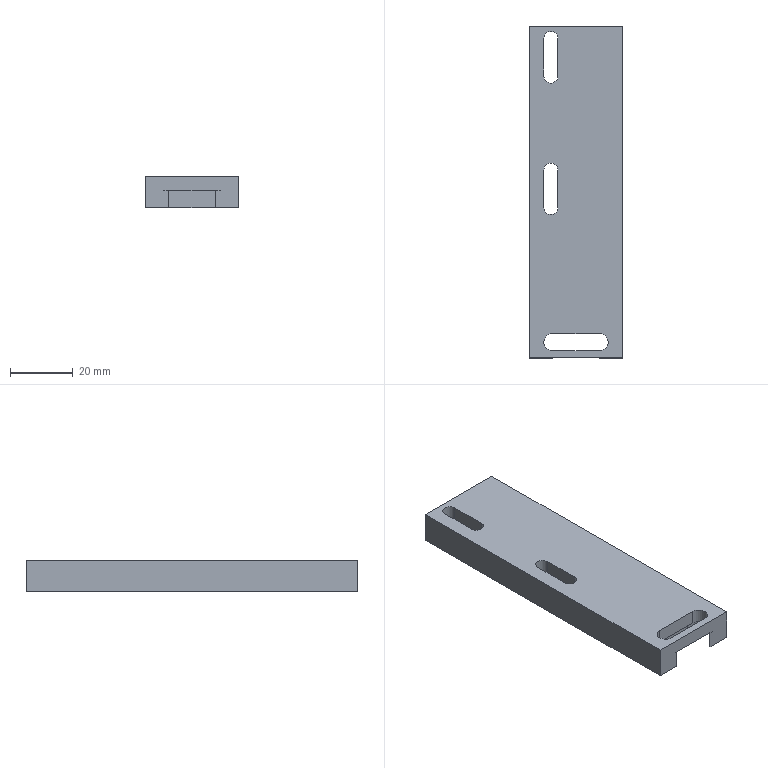Part | NX | 1 solid | 22 faces | box 30 x 106 x 10 mm | volume 28667 mm3 | plane 14 | cylinder 8 | commonest cylinder face diameters 4.5 x4 5.5 x2 10 x2
STEP:
#1=CARTESIAN_POINT('',(-10.25,49.,0.));
#2=VERTEX_POINT('',#1);
#3=CARTESIAN_POINT('',(-10.25,37.,0.));
#4=VERTEX_POINT('',#3);
#5=CARTESIAN_POINT('',(-10.25,0.,0.));
#6=DIRECTION('',(0.,-1.,0.));
#7=VECTOR('',#6,1000.);
#8=LINE('',#5,#7);
#9=EDGE_CURVE('',#2,#4,#8,.T.);
#10=ORIENTED_EDGE('',*,*,#9,.T.);
#11=CARTESIAN_POINT('',(-5.75,37.,0.));
#12=VERTEX_POINT('',#11);
#13=CARTESIAN_POINT('',(-8.,37.,0.));
#14=DIRECTION('',(0.,0.,1.));
#15=DIRECTION('',(1.,0.,0.));
#16=AXIS2_PLACEMENT_3D('',#13,#14,#15);
#17=CIRCLE('',#16,2.25);
#18=EDGE_CURVE('',#4,#12,#17,.T.);
#19=ORIENTED_EDGE('',*,*,#18,.T.);
#20=CARTESIAN_POINT('',(-5.75,49.,0.));
#21=VERTEX_POINT('',#20);
#22=CARTESIAN_POINT('',(-5.75,0.,0.));
#23=DIRECTION('',(0.,1.,0.));
#24=VECTOR('',#23,1000.);
#25=LINE('',#22,#24);
#26=EDGE_CURVE('',#12,#21,#25,.T.);
#27=ORIENTED_EDGE('',*,*,#26,.T.);
#28=CARTESIAN_POINT('',(-8.,49.,0.));
#29=DIRECTION('',(0.,0.,1.));
#30=DIRECTION('',(-1.,0.,0.));
#31=AXIS2_PLACEMENT_3D('',#28,#29,#30);
#32=CIRCLE('',#31,2.25);
#33=EDGE_CURVE('',#21,#2,#32,.T.);
#34=ORIENTED_EDGE('',*,*,#33,.T.);
#35=EDGE_LOOP('',(#10,#19,#27,#34));
#36=FACE_BOUND('',#35,.T.);
#37=CARTESIAN_POINT('',(-10.25,-5.,0.));
#38=VERTEX_POINT('',#37);
#39=CARTESIAN_POINT('',(-5.75,-5.,0.));
#40=VERTEX_POINT('',#39);
#41=CARTESIAN_POINT('',(-8.,-5.,0.));
#42=DIRECTION('',(0.,0.,1.));
#43=DIRECTION('',(1.,0.,0.));
#44=AXIS2_PLACEMENT_3D('',#41,#42,#43);
#45=CIRCLE('',#44,2.25);
#46=EDGE_CURVE('',#38,#40,#45,.T.);
#47=ORIENTED_EDGE('',*,*,#46,.T.);
#48=CARTESIAN_POINT('',(-5.75,7.,0.));
#49=VERTEX_POINT('',#48);
#50=CARTESIAN_POINT('',(-5.75,-2.5,0.));
#51=DIRECTION('',(0.,1.,0.));
#52=VECTOR('',#51,1000.);
#53=LINE('',#50,#52);
#54=EDGE_CURVE('',#40,#49,#53,.T.);
#55=ORIENTED_EDGE('',*,*,#54,.T.);
#56=CARTESIAN_POINT('',(-10.25,7.,0.));
#57=VERTEX_POINT('',#56);
#58=CARTESIAN_POINT('',(-8.,7.,0.));
#59=DIRECTION('',(0.,0.,1.));
#60=DIRECTION('',(-1.,0.,0.));
#61=AXIS2_PLACEMENT_3D('',#58,#59,#60);
#62=CIRCLE('',#61,2.25);
#63=EDGE_CURVE('',#49,#57,#62,.T.);
#64=ORIENTED_EDGE('',*,*,#63,.T.);
#65=CARTESIAN_POINT('',(-10.25,3.5,0.));
#66=DIRECTION('',(0.,-1.,0.));
#67=VECTOR('',#66,1000.);
#68=LINE('',#65,#67);
#69=EDGE_CURVE('',#57,#38,#68,.T.);
#70=ORIENTED_EDGE('',*,*,#69,.T.);
#71=EDGE_LOOP('',(#47,#55,#64,#70));
#72=FACE_BOUND('',#71,.T.);
#73=CARTESIAN_POINT('',(-7.5,-43.,0.));
#74=VERTEX_POINT('',#73);
#75=CARTESIAN_POINT('',(-7.5,-53.,0.));
#76=VERTEX_POINT('',#75);
#77=CARTESIAN_POINT('',(-7.5,-48.,0.));
#78=DIRECTION('',(0.,0.,1.));
#79=DIRECTION('',(0.,-1.,0.));
#80=AXIS2_PLACEMENT_3D('',#77,#78,#79);
#81=CIRCLE('',#80,5.);
#82=EDGE_CURVE('',#74,#76,#81,.T.);
#83=ORIENTED_EDGE('',*,*,#82,.T.);
#84=CARTESIAN_POINT('',(-15.,-53.,0.));
#85=VERTEX_POINT('',#84);
#86=CARTESIAN_POINT('',(-15.,-53.,0.));
#87=DIRECTION('',(1.,0.,0.));
#88=VECTOR('',#87,1000.);
#89=LINE('',#86,#88);
#90=EDGE_CURVE('',#85,#76,#89,.T.);
#91=ORIENTED_EDGE('',*,*,#90,.F.);
#92=CARTESIAN_POINT('',(-15.,53.,0.));
#93=VERTEX_POINT('',#92);
#94=CARTESIAN_POINT('',(-15.,53.,0.));
#95=DIRECTION('',(0.,-1.,0.));
#96=VECTOR('',#95,1000.);
#97=LINE('',#94,#96);
#98=EDGE_CURVE('',#93,#85,#97,.T.);
#99=ORIENTED_EDGE('',*,*,#98,.F.);
#100=CARTESIAN_POINT('',(15.,53.,0.));
#101=VERTEX_POINT('',#100);
#102=CARTESIAN_POINT('',(15.,53.,0.));
#103=DIRECTION('',(-1.,0.,0.));
#104=VECTOR('',#103,1000.);
#105=LINE('',#102,#104);
#106=EDGE_CURVE('',#101,#93,#105,.T.);
#107=ORIENTED_EDGE('',*,*,#106,.F.);
#108=CARTESIAN_POINT('',(15.,-53.,0.));
#109=VERTEX_POINT('',#108);
#110=CARTESIAN_POINT('',(15.,-53.,0.));
#111=DIRECTION('',(0.,1.,0.));
#112=VECTOR('',#111,1000.);
#113=LINE('',#110,#112);
#114=EDGE_CURVE('',#109,#101,#113,.T.);
#115=ORIENTED_EDGE('',*,*,#114,.F.);
#116=CARTESIAN_POINT('',(7.5,-53.,0.));
#117=VERTEX_POINT('',#116);
#118=CARTESIAN_POINT('',(-15.,-53.,0.));
#119=DIRECTION('',(1.,0.,0.));
#120=VECTOR('',#119,1000.);
#121=LINE('',#118,#120);
#122=EDGE_CURVE('',#117,#109,#121,.T.);
#123=ORIENTED_EDGE('',*,*,#122,.F.);
#124=CARTESIAN_POINT('',(7.5,-43.,0.));
#125=VERTEX_POINT('',#124);
#126=CARTESIAN_POINT('',(7.5,-48.,0.));
#127=DIRECTION('',(0.,0.,1.));
#128=DIRECTION('',(0.,1.,0.));
#129=AXIS2_PLACEMENT_3D('',#126,#127,#128);
#130=CIRCLE('',#129,5.);
#131=EDGE_CURVE('',#117,#125,#130,.T.);
#132=ORIENTED_EDGE('',*,*,#131,.T.);
#133=CARTESIAN_POINT('',(3.75,-43.,0.));
#134=DIRECTION('',(-1.,0.,0.));
#135=VECTOR('',#134,1000.);
#136=LINE('',#133,#135);
#137=EDGE_CURVE('',#125,#74,#136,.T.);
#138=ORIENTED_EDGE('',*,*,#137,.T.);
#139=EDGE_LOOP('',(#83,#91,#99,#107,#115,#123,#132,#138));
#140=FACE_BOUND('',#139,.T.);
#141=CARTESIAN_POINT('',(0.,0.,0.));
#142=DIRECTION('',(0.,0.,1.));
#143=DIRECTION('',(1.,0.,0.));
#144=AXIS2_PLACEMENT_3D('',#141,#142,#143);
#145=PLANE('',#144);
#146=ADVANCED_FACE('',(#36,#72,#140),#145,.F.);
#147=CARTESIAN_POINT('',(-10.25,37.,10.));
#148=VERTEX_POINT('',#147);
#149=CARTESIAN_POINT('',(-10.25,49.,10.));
#150=VERTEX_POINT('',#149);
#151=CARTESIAN_POINT('',(-10.25,0.,10.));
#152=DIRECTION('',(0.,1.,0.));
#153=VECTOR('',#152,1000.);
#154=LINE('',#151,#153);
#155=EDGE_CURVE('',#148,#150,#154,.T.);
#156=ORIENTED_EDGE('',*,*,#155,.T.);
#157=CARTESIAN_POINT('',(-5.75,49.,10.));
#158=VERTEX_POINT('',#157);
#159=CARTESIAN_POINT('',(-8.,49.,10.));
#160=DIRECTION('',(0.,0.,-1.));
#161=DIRECTION('',(-1.,0.,0.));
#162=AXIS2_PLACEMENT_3D('',#159,#160,#161);
#163=CIRCLE('',#162,2.25);
#164=EDGE_CURVE('',#150,#158,#163,.T.);
#165=ORIENTED_EDGE('',*,*,#164,.T.);
#166=CARTESIAN_POINT('',(-5.75,37.,10.));
#167=VERTEX_POINT('',#166);
#168=CARTESIAN_POINT('',(-5.75,0.,10.));
#169=DIRECTION('',(0.,-1.,0.));
#170=VECTOR('',#169,1000.);
#171=LINE('',#168,#170);
#172=EDGE_CURVE('',#158,#167,#171,.T.);
#173=ORIENTED_EDGE('',*,*,#172,.T.);
#174=CARTESIAN_POINT('',(-8.,37.,10.));
#175=DIRECTION('',(0.,0.,-1.));
#176=DIRECTION('',(1.,0.,0.));
#177=AXIS2_PLACEMENT_3D('',#174,#175,#176);
#178=CIRCLE('',#177,2.25);
#179=EDGE_CURVE('',#167,#148,#178,.T.);
#180=ORIENTED_EDGE('',*,*,#179,.T.);
#181=EDGE_LOOP('',(#156,#165,#173,#180));
#182=FACE_BOUND('',#181,.T.);
#183=CARTESIAN_POINT('',(-5.75,-5.,10.));
#184=VERTEX_POINT('',#183);
#185=CARTESIAN_POINT('',(-10.25,-5.,10.));
#186=VERTEX_POINT('',#185);
#187=CARTESIAN_POINT('',(-8.,-5.,10.));
#188=DIRECTION('',(0.,0.,-1.));
#189=DIRECTION('',(1.,0.,0.));
#190=AXIS2_PLACEMENT_3D('',#187,#188,#189);
#191=CIRCLE('',#190,2.25);
#192=EDGE_CURVE('',#184,#186,#191,.T.);
#193=ORIENTED_EDGE('',*,*,#192,.T.);
#194=CARTESIAN_POINT('',(-10.25,7.,10.));
#195=VERTEX_POINT('',#194);
#196=CARTESIAN_POINT('',(-10.25,3.5,10.));
#197=DIRECTION('',(0.,1.,0.));
#198=VECTOR('',#197,1000.);
#199=LINE('',#196,#198);
#200=EDGE_CURVE('',#186,#195,#199,.T.);
#201=ORIENTED_EDGE('',*,*,#200,.T.);
#202=CARTESIAN_POINT('',(-5.75,7.,10.));
#203=VERTEX_POINT('',#202);
#204=CARTESIAN_POINT('',(-8.,7.,10.));
#205=DIRECTION('',(0.,0.,-1.));
#206=DIRECTION('',(-1.,0.,0.));
#207=AXIS2_PLACEMENT_3D('',#204,#205,#206);
#208=CIRCLE('',#207,2.25);
#209=EDGE_CURVE('',#195,#203,#208,.T.);
#210=ORIENTED_EDGE('',*,*,#209,.T.);
#211=CARTESIAN_POINT('',(-5.75,-2.5,10.));
#212=DIRECTION('',(0.,-1.,0.));
#213=VECTOR('',#212,1000.);
#214=LINE('',#211,#213);
#215=EDGE_CURVE('',#203,#184,#214,.T.);
#216=ORIENTED_EDGE('',*,*,#215,.T.);
#217=EDGE_LOOP('',(#193,#201,#210,#216));
#218=FACE_BOUND('',#217,.T.);
#219=CARTESIAN_POINT('',(-7.5,-45.25,10.));
#220=VERTEX_POINT('',#219);
#221=CARTESIAN_POINT('',(7.5,-45.25,10.));
#222=VERTEX_POINT('',#221);
#223=CARTESIAN_POINT('',(3.75,-45.25,10.));
#224=DIRECTION('',(1.,0.,0.));
#225=VECTOR('',#224,1000.);
#226=LINE('',#223,#225);
#227=EDGE_CURVE('',#220,#222,#226,.T.);
#228=ORIENTED_EDGE('',*,*,#227,.T.);
#229=CARTESIAN_POINT('',(7.5,-50.75,10.));
#230=VERTEX_POINT('',#229);
#231=CARTESIAN_POINT('',(7.5,-48.,10.));
#232=DIRECTION('',(0.,0.,-1.));
#233=DIRECTION('',(0.,1.,0.));
#234=AXIS2_PLACEMENT_3D('',#231,#232,#233);
#235=CIRCLE('',#234,2.75);
#236=EDGE_CURVE('',#222,#230,#235,.T.);
#237=ORIENTED_EDGE('',*,*,#236,.T.);
#238=CARTESIAN_POINT('',(-7.5,-50.75,10.));
#239=VERTEX_POINT('',#238);
#240=CARTESIAN_POINT('',(-3.75,-50.75,10.));
#241=DIRECTION('',(-1.,0.,0.));
#242=VECTOR('',#241,1000.);
#243=LINE('',#240,#242);
#244=EDGE_CURVE('',#230,#239,#243,.T.);
#245=ORIENTED_EDGE('',*,*,#244,.T.);
#246=CARTESIAN_POINT('',(-7.5,-48.,10.));
#247=DIRECTION('',(0.,0.,-1.));
#248=DIRECTION('',(0.,-1.,0.));
#249=AXIS2_PLACEMENT_3D('',#246,#247,#248);
#250=CIRCLE('',#249,2.75);
#251=EDGE_CURVE('',#239,#220,#250,.T.);
#252=ORIENTED_EDGE('',*,*,#251,.T.);
#253=EDGE_LOOP('',(#228,#237,#245,#252));
#254=FACE_BOUND('',#253,.T.);
#255=CARTESIAN_POINT('',(15.,-53.,10.));
#256=VERTEX_POINT('',#255);
#257=CARTESIAN_POINT('',(15.,53.,10.));
#258=VERTEX_POINT('',#257);
#259=CARTESIAN_POINT('',(15.,-53.,10.));
#260=DIRECTION('',(0.,1.,0.));
#261=VECTOR('',#260,1000.);
#262=LINE('',#259,#261);
#263=EDGE_CURVE('',#256,#258,#262,.T.);
#264=ORIENTED_EDGE('',*,*,#263,.T.);
#265=CARTESIAN_POINT('',(-15.,53.,10.));
#266=VERTEX_POINT('',#265);
#267=CARTESIAN_POINT('',(15.,53.,10.));
#268=DIRECTION('',(-1.,0.,0.));
#269=VECTOR('',#268,1000.);
#270=LINE('',#267,#269);
#271=EDGE_CURVE('',#258,#266,#270,.T.);
#272=ORIENTED_EDGE('',*,*,#271,.T.);
#273=CARTESIAN_POINT('',(-15.,-53.,10.));
#274=VERTEX_POINT('',#273);
#275=CARTESIAN_POINT('',(-15.,53.,10.));
#276=DIRECTION('',(0.,-1.,0.));
#277=VECTOR('',#276,1000.);
#278=LINE('',#275,#277);
#279=EDGE_CURVE('',#266,#274,#278,.T.);
#280=ORIENTED_EDGE('',*,*,#279,.T.);
#281=CARTESIAN_POINT('',(-15.,-53.,10.));
#282=DIRECTION('',(1.,0.,0.));
#283=VECTOR('',#282,1000.);
#284=LINE('',#281,#283);
#285=EDGE_CURVE('',#274,#256,#284,.T.);
#286=ORIENTED_EDGE('',*,*,#285,.T.);
#287=EDGE_LOOP('',(#264,#272,#280,#286));
#288=FACE_BOUND('',#287,.T.);
#289=CARTESIAN_POINT('',(0.,0.,10.));
#290=DIRECTION('',(0.,0.,1.));
#291=DIRECTION('',(1.,0.,0.));
#292=AXIS2_PLACEMENT_3D('',#289,#290,#291);
#293=PLANE('',#292);
#294=ADVANCED_FACE('',(#182,#218,#254,#288),#293,.T.);
#295=ORIENTED_EDGE('',*,*,#114,.T.);
#296=CARTESIAN_POINT('',(15.,53.,0.));
#297=DIRECTION('',(0.,0.,1.));
#298=VECTOR('',#297,1000.);
#299=LINE('',#296,#298);
#300=EDGE_CURVE('',#101,#258,#299,.T.);
#301=ORIENTED_EDGE('',*,*,#300,.T.);
#302=ORIENTED_EDGE('',*,*,#263,.F.);
#303=CARTESIAN_POINT('',(15.,-53.,0.));
#304=DIRECTION('',(0.,0.,1.));
#305=VECTOR('',#304,1000.);
#306=LINE('',#303,#305);
#307=EDGE_CURVE('',#109,#256,#306,.T.);
#308=ORIENTED_EDGE('',*,*,#307,.F.);
#309=EDGE_LOOP('',(#295,#301,#302,#308));
#310=FACE_BOUND('',#309,.T.);
#311=CARTESIAN_POINT('',(15.,-53.,0.));
#312=DIRECTION('',(1.,0.,0.));
#313=DIRECTION('',(0.,1.,0.));
#314=AXIS2_PLACEMENT_3D('',#311,#312,#313);
#315=PLANE('',#314);
#316=ADVANCED_FACE('',(#310),#315,.T.);
#317=ORIENTED_EDGE('',*,*,#106,.T.);
#318=CARTESIAN_POINT('',(-15.,53.,0.));
#319=DIRECTION('',(0.,0.,1.));
#320=VECTOR('',#319,1000.);
#321=LINE('',#318,#320);
#322=EDGE_CURVE('',#93,#266,#321,.T.);
#323=ORIENTED_EDGE('',*,*,#322,.T.);
#324=ORIENTED_EDGE('',*,*,#271,.F.);
#325=ORIENTED_EDGE('',*,*,#300,.F.);
#326=EDGE_LOOP('',(#317,#323,#324,#325));
#327=FACE_BOUND('',#326,.T.);
#328=CARTESIAN_POINT('',(15.,53.,0.));
#329=DIRECTION('',(0.,1.,0.));
#330=DIRECTION('',(-1.,0.,0.));
#331=AXIS2_PLACEMENT_3D('',#328,#329,#330);
#332=PLANE('',#331);
#333=ADVANCED_FACE('',(#327),#332,.T.);
#334=ORIENTED_EDGE('',*,*,#98,.T.);
#335=CARTESIAN_POINT('',(-15.,-53.,0.));
#336=DIRECTION('',(0.,0.,1.));
#337=VECTOR('',#336,1000.);
#338=LINE('',#335,#337);
#339=EDGE_CURVE('',#85,#274,#338,.T.);
#340=ORIENTED_EDGE('',*,*,#339,.T.);
#341=ORIENTED_EDGE('',*,*,#279,.F.);
#342=ORIENTED_EDGE('',*,*,#322,.F.);
#343=EDGE_LOOP('',(#334,#340,#341,#342));
#344=FACE_BOUND('',#343,.T.);
#345=CARTESIAN_POINT('',(-15.,53.,0.));
#346=DIRECTION('',(-1.,0.,0.));
#347=DIRECTION('',(0.,-1.,0.));
#348=AXIS2_PLACEMENT_3D('',#345,#346,#347);
#349=PLANE('',#348);
#350=ADVANCED_FACE('',(#344),#349,.T.);
#351=ORIENTED_EDGE('',*,*,#164,.F.);
#352=CARTESIAN_POINT('',(-10.25,49.,0.));
#353=DIRECTION('',(0.,0.,1.));
#354=VECTOR('',#353,1000.);
#355=LINE('',#352,#354);
#356=EDGE_CURVE('',#2,#150,#355,.T.);
#357=ORIENTED_EDGE('',*,*,#356,.F.);
#358=ORIENTED_EDGE('',*,*,#33,.F.);
#359=CARTESIAN_POINT('',(-5.75,49.,0.));
#360=DIRECTION('',(0.,0.,1.));
#361=VECTOR('',#360,1000.);
#362=LINE('',#359,#361);
#363=EDGE_CURVE('',#21,#158,#362,.T.);
#364=ORIENTED_EDGE('',*,*,#363,.T.);
#365=EDGE_LOOP('',(#351,#357,#358,#364));
#366=FACE_BOUND('',#365,.T.);
#367=CARTESIAN_POINT('',(-8.,49.,0.));
#368=DIRECTION('',(0.,0.,1.));
#369=DIRECTION('',(-1.,0.,0.));
#370=AXIS2_PLACEMENT_3D('',#367,#368,#369);
#371=CYLINDRICAL_SURFACE('',#370,2.25);
#372=ADVANCED_FACE('',(#366),#371,.F.);
#373=ORIENTED_EDGE('',*,*,#155,.F.);
#374=CARTESIAN_POINT('',(-10.25,37.,0.));
#375=DIRECTION('',(0.,0.,1.));
#376=VECTOR('',#375,1000.);
#377=LINE('',#374,#376);
#378=EDGE_CURVE('',#4,#148,#377,.T.);
#379=ORIENTED_EDGE('',*,*,#378,.F.);
#380=ORIENTED_EDGE('',*,*,#9,.F.);
#381=ORIENTED_EDGE('',*,*,#356,.T.);
#382=EDGE_LOOP('',(#373,#379,#380,#381));
#383=FACE_BOUND('',#382,.T.);
#384=CARTESIAN_POINT('',(-10.25,7.,0.));
#385=DIRECTION('',(-1.,0.,0.));
#386=DIRECTION('',(0.,-1.,0.));
#387=AXIS2_PLACEMENT_3D('',#384,#385,#386);
#388=PLANE('',#387);
#389=ADVANCED_FACE('',(#383),#388,.F.);
#390=ORIENTED_EDGE('',*,*,#179,.F.);
#391=CARTESIAN_POINT('',(-5.75,37.,0.));
#392=DIRECTION('',(0.,0.,1.));
#393=VECTOR('',#392,1000.);
#394=LINE('',#391,#393);
#395=EDGE_CURVE('',#12,#167,#394,.T.);
#396=ORIENTED_EDGE('',*,*,#395,.F.);
#397=ORIENTED_EDGE('',*,*,#18,.F.);
#398=ORIENTED_EDGE('',*,*,#378,.T.);
#399=EDGE_LOOP('',(#390,#396,#397,#398));
#400=FACE_BOUND('',#399,.T.);
#401=CARTESIAN_POINT('',(-8.,37.,0.));
#402=DIRECTION('',(0.,0.,1.));
#403=DIRECTION('',(1.,0.,0.));
#404=AXIS2_PLACEMENT_3D('',#401,#402,#403);
#405=CYLINDRICAL_SURFACE('',#404,2.25);
#406=ADVANCED_FACE('',(#400),#405,.F.);
#407=ORIENTED_EDGE('',*,*,#172,.F.);
#408=ORIENTED_EDGE('',*,*,#363,.F.);
#409=ORIENTED_EDGE('',*,*,#26,.F.);
#410=ORIENTED_EDGE('',*,*,#395,.T.);
#411=EDGE_LOOP('',(#407,#408,#409,#410));
#412=FACE_BOUND('',#411,.T.);
#413=CARTESIAN_POINT('',(-5.75,-5.,0.));
#414=DIRECTION('',(1.,0.,0.));
#415=DIRECTION('',(0.,1.,0.));
#416=AXIS2_PLACEMENT_3D('',#413,#414,#415);
#417=PLANE('',#416);
#418=ADVANCED_FACE('',(#412),#417,.F.);
#419=ORIENTED_EDGE('',*,*,#200,.F.);
#420=CARTESIAN_POINT('',(-10.25,-5.,0.));
#421=DIRECTION('',(0.,0.,1.));
#422=VECTOR('',#421,1000.);
#423=LINE('',#420,#422);
#424=EDGE_CURVE('',#38,#186,#423,.T.);
#425=ORIENTED_EDGE('',*,*,#424,.F.);
#426=ORIENTED_EDGE('',*,*,#69,.F.);
#427=CARTESIAN_POINT('',(-10.25,7.,0.));
#428=DIRECTION('',(0.,0.,1.));
#429=VECTOR('',#428,1000.);
#430=LINE('',#427,#429);
#431=EDGE_CURVE('',#57,#195,#430,.T.);
#432=ORIENTED_EDGE('',*,*,#431,.T.);
#433=EDGE_LOOP('',(#419,#425,#426,#432));
#434=FACE_BOUND('',#433,.T.);
#435=CARTESIAN_POINT('',(-10.25,7.,0.));
#436=DIRECTION('',(-1.,0.,0.));
#437=DIRECTION('',(0.,-1.,0.));
#438=AXIS2_PLACEMENT_3D('',#435,#436,#437);
#439=PLANE('',#438);
#440=ADVANCED_FACE('',(#434),#439,.F.);
#441=ORIENTED_EDGE('',*,*,#192,.F.);
#442=CARTESIAN_POINT('',(-5.75,-5.,0.));
#443=DIRECTION('',(0.,0.,1.));
#444=VECTOR('',#443,1000.);
#445=LINE('',#442,#444);
#446=EDGE_CURVE('',#40,#184,#445,.T.);
#447=ORIENTED_EDGE('',*,*,#446,.F.);
#448=ORIENTED_EDGE('',*,*,#46,.F.);
#449=ORIENTED_EDGE('',*,*,#424,.T.);
#450=EDGE_LOOP('',(#441,#447,#448,#449));
#451=FACE_BOUND('',#450,.T.);
#452=CARTESIAN_POINT('',(-8.,-5.,0.));
#453=DIRECTION('',(0.,0.,1.));
#454=DIRECTION('',(1.,0.,0.));
#455=AXIS2_PLACEMENT_3D('',#452,#453,#454);
#456=CYLINDRICAL_SURFACE('',#455,2.25);
#457=ADVANCED_FACE('',(#451),#456,.F.);
#458=ORIENTED_EDGE('',*,*,#215,.F.);
#459=CARTESIAN_POINT('',(-5.75,7.,0.));
#460=DIRECTION('',(0.,0.,1.));
#461=VECTOR('',#460,1000.);
#462=LINE('',#459,#461);
#463=EDGE_CURVE('',#49,#203,#462,.T.);
#464=ORIENTED_EDGE('',*,*,#463,.F.);
#465=ORIENTED_EDGE('',*,*,#54,.F.);
#466=ORIENTED_EDGE('',*,*,#446,.T.);
#467=EDGE_LOOP('',(#458,#464,#465,#466));
#468=FACE_BOUND('',#467,.T.);
#469=CARTESIAN_POINT('',(-5.75,-5.,0.));
#470=DIRECTION('',(1.,0.,0.));
#471=DIRECTION('',(0.,1.,0.));
#472=AXIS2_PLACEMENT_3D('',#469,#470,#471);
#473=PLANE('',#472);
#474=ADVANCED_FACE('',(#468),#473,.F.);
#475=ORIENTED_EDGE('',*,*,#209,.F.);
#476=ORIENTED_EDGE('',*,*,#431,.F.);
#477=ORIENTED_EDGE('',*,*,#63,.F.);
#478=ORIENTED_EDGE('',*,*,#463,.T.);
#479=EDGE_LOOP('',(#475,#476,#477,#478));
#480=FACE_BOUND('',#479,.T.);
#481=CARTESIAN_POINT('',(-8.,7.,0.));
#482=DIRECTION('',(0.,0.,1.));
#483=DIRECTION('',(-1.,0.,0.));
#484=AXIS2_PLACEMENT_3D('',#481,#482,#483);
#485=CYLINDRICAL_SURFACE('',#484,2.25);
#486=ADVANCED_FACE('',(#480),#485,.F.);
#487=CARTESIAN_POINT('',(-7.5,-50.75,5.5));
#488=VERTEX_POINT('',#487);
#489=CARTESIAN_POINT('',(-7.5,-45.25,5.5));
#490=VERTEX_POINT('',#489);
#491=CARTESIAN_POINT('',(-7.5,-48.,5.5));
#492=DIRECTION('',(0.,0.,-1.));
#493=DIRECTION('',(0.,-1.,0.));
#494=AXIS2_PLACEMENT_3D('',#491,#492,#493);
#495=CIRCLE('',#494,2.75);
#496=EDGE_CURVE('',#488,#490,#495,.T.);
#497=ORIENTED_EDGE('',*,*,#496,.T.);
#498=CARTESIAN_POINT('',(-7.5,-45.25,0.));
#499=DIRECTION('',(0.,0.,1.));
#500=VECTOR('',#499,1000.);
#501=LINE('',#498,#500);
#502=EDGE_CURVE('',#490,#220,#501,.T.);
#503=ORIENTED_EDGE('',*,*,#502,.T.);
#504=ORIENTED_EDGE('',*,*,#251,.F.);
#505=CARTESIAN_POINT('',(-7.5,-50.75,0.));
#506=DIRECTION('',(0.,0.,1.));
#507=VECTOR('',#506,1000.);
#508=LINE('',#505,#507);
#509=EDGE_CURVE('',#488,#239,#508,.T.);
#510=ORIENTED_EDGE('',*,*,#509,.F.);
#511=EDGE_LOOP('',(#497,#503,#504,#510));
#512=FACE_BOUND('',#511,.T.);
#513=CARTESIAN_POINT('',(-7.5,-48.,0.));
#514=DIRECTION('',(0.,0.,1.));
#515=DIRECTION('',(0.,-1.,0.));
#516=AXIS2_PLACEMENT_3D('',#513,#514,#515);
#517=CYLINDRICAL_SURFACE('',#516,2.75);
#518=ADVANCED_FACE('',(#512),#517,.F.);
#519=CARTESIAN_POINT('',(7.5,-50.75,5.5));
#520=VERTEX_POINT('',#519);
#521=CARTESIAN_POINT('',(-3.75,-50.75,5.5));
#522=DIRECTION('',(-1.,0.,0.));
#523=VECTOR('',#522,1000.);
#524=LINE('',#521,#523);
#525=EDGE_CURVE('',#520,#488,#524,.T.);
#526=ORIENTED_EDGE('',*,*,#525,.T.);
#527=ORIENTED_EDGE('',*,*,#509,.T.);
#528=ORIENTED_EDGE('',*,*,#244,.F.);
#529=CARTESIAN_POINT('',(7.5,-50.75,0.));
#530=DIRECTION('',(0.,0.,1.));
#531=VECTOR('',#530,1000.);
#532=LINE('',#529,#531);
#533=EDGE_CURVE('',#520,#230,#532,.T.);
#534=ORIENTED_EDGE('',*,*,#533,.F.);
#535=EDGE_LOOP('',(#526,#527,#528,#534));
#536=FACE_BOUND('',#535,.T.);
#537=CARTESIAN_POINT('',(-7.5,-50.75,0.));
#538=DIRECTION('',(0.,-1.,0.));
#539=DIRECTION('',(1.,0.,0.));
#540=AXIS2_PLACEMENT_3D('',#537,#538,#539);
#541=PLANE('',#540);
#542=ADVANCED_FACE('',(#536),#541,.F.);
#543=CARTESIAN_POINT('',(7.5,-45.25,5.5));
#544=VERTEX_POINT('',#543);
#545=CARTESIAN_POINT('',(7.5,-48.,5.5));
#546=DIRECTION('',(0.,0.,-1.));
#547=DIRECTION('',(0.,1.,0.));
#548=AXIS2_PLACEMENT_3D('',#545,#546,#547);
#549=CIRCLE('',#548,2.75);
#550=EDGE_CURVE('',#544,#520,#549,.T.);
#551=ORIENTED_EDGE('',*,*,#550,.T.);
#552=ORIENTED_EDGE('',*,*,#533,.T.);
#553=ORIENTED_EDGE('',*,*,#236,.F.);
#554=CARTESIAN_POINT('',(7.5,-45.25,0.));
#555=DIRECTION('',(0.,0.,1.));
#556=VECTOR('',#555,1000.);
#557=LINE('',#554,#556);
#558=EDGE_CURVE('',#544,#222,#557,.T.);
#559=ORIENTED_EDGE('',*,*,#558,.F.);
#560=EDGE_LOOP('',(#551,#552,#553,#559));
#561=FACE_BOUND('',#560,.T.);
#562=CARTESIAN_POINT('',(7.5,-48.,0.));
#563=DIRECTION('',(0.,0.,1.));
#564=DIRECTION('',(0.,1.,0.));
#565=AXIS2_PLACEMENT_3D('',#562,#563,#564);
#566=CYLINDRICAL_SURFACE('',#565,2.75);
#567=ADVANCED_FACE('',(#561),#566,.F.);
#568=CARTESIAN_POINT('',(3.75,-45.25,5.5));
#569=DIRECTION('',(1.,0.,0.));
#570=VECTOR('',#569,1000.);
#571=LINE('',#568,#570);
#572=EDGE_CURVE('',#490,#544,#571,.T.);
#573=ORIENTED_EDGE('',*,*,#572,.T.);
#574=ORIENTED_EDGE('',*,*,#558,.T.);
#575=ORIENTED_EDGE('',*,*,#227,.F.);
#576=ORIENTED_EDGE('',*,*,#502,.F.);
#577=EDGE_LOOP('',(#573,#574,#575,#576));
#578=FACE_BOUND('',#577,.T.);
#579=CARTESIAN_POINT('',(7.5,-45.25,0.));
#580=DIRECTION('',(0.,1.,0.));
#581=DIRECTION('',(-1.,0.,0.));
#582=AXIS2_PLACEMENT_3D('',#579,#580,#581);
#583=PLANE('',#582);
#584=ADVANCED_FACE('',(#578),#583,.F.);
#585=CARTESIAN_POINT('',(-7.5,-53.,5.5));
#586=VERTEX_POINT('',#585);
#587=CARTESIAN_POINT('',(-7.5,-53.,0.));
#588=DIRECTION('',(0.,0.,1.));
#589=VECTOR('',#588,1000.);
#590=LINE('',#587,#589);
#591=EDGE_CURVE('',#76,#586,#590,.T.);
#592=ORIENTED_EDGE('',*,*,#591,.T.);
#593=CARTESIAN_POINT('',(7.5,-53.,5.5));
#594=VERTEX_POINT('',#593);
#595=CARTESIAN_POINT('',(-7.5,-53.,5.5));
#596=DIRECTION('',(1.,0.,0.));
#597=VECTOR('',#596,1000.);
#598=LINE('',#595,#597);
#599=EDGE_CURVE('',#586,#594,#598,.T.);
#600=ORIENTED_EDGE('',*,*,#599,.T.);
#601=CARTESIAN_POINT('',(7.5,-53.,0.));
#602=DIRECTION('',(0.,0.,1.));
#603=VECTOR('',#602,1000.);
#604=LINE('',#601,#603);
#605=EDGE_CURVE('',#117,#594,#604,.T.);
#606=ORIENTED_EDGE('',*,*,#605,.F.);
#607=ORIENTED_EDGE('',*,*,#122,.T.);
#608=ORIENTED_EDGE('',*,*,#307,.T.);
#609=ORIENTED_EDGE('',*,*,#285,.F.);
#610=ORIENTED_EDGE('',*,*,#339,.F.);
#611=ORIENTED_EDGE('',*,*,#90,.T.);
#612=EDGE_LOOP('',(#592,#600,#606,#607,#608,#609,#610,#611));
#613=FACE_BOUND('',#612,.T.);
#614=CARTESIAN_POINT('',(-15.,-53.,0.));
#615=DIRECTION('',(0.,-1.,0.));
#616=DIRECTION('',(1.,0.,0.));
#617=AXIS2_PLACEMENT_3D('',#614,#615,#616);
#618=PLANE('',#617);
#619=ADVANCED_FACE('',(#613),#618,.T.);
#620=ORIENTED_EDGE('',*,*,#525,.F.);
#621=ORIENTED_EDGE('',*,*,#550,.F.);
#622=ORIENTED_EDGE('',*,*,#572,.F.);
#623=ORIENTED_EDGE('',*,*,#496,.F.);
#624=EDGE_LOOP('',(#620,#621,#622,#623));
#625=FACE_BOUND('',#624,.T.);
#626=CARTESIAN_POINT('',(-7.5,-43.,5.5));
#627=VERTEX_POINT('',#626);
#628=CARTESIAN_POINT('',(-7.5,-48.,5.5));
#629=DIRECTION('',(0.,0.,1.));
#630=DIRECTION('',(0.,-1.,0.));
#631=AXIS2_PLACEMENT_3D('',#628,#629,#630);
#632=CIRCLE('',#631,5.);
#633=EDGE_CURVE('',#627,#586,#632,.T.);
#634=ORIENTED_EDGE('',*,*,#633,.F.);
#635=CARTESIAN_POINT('',(7.5,-43.,5.5));
#636=VERTEX_POINT('',#635);
#637=CARTESIAN_POINT('',(-7.5,-43.,5.5));
#638=DIRECTION('',(-1.,0.,0.));
#639=VECTOR('',#638,1000.);
#640=LINE('',#637,#639);
#641=EDGE_CURVE('',#636,#627,#640,.T.);
#642=ORIENTED_EDGE('',*,*,#641,.F.);
#643=CARTESIAN_POINT('',(7.5,-48.,5.5));
#644=DIRECTION('',(0.,0.,1.));
#645=DIRECTION('',(0.,1.,0.));
#646=AXIS2_PLACEMENT_3D('',#643,#644,#645);
#647=CIRCLE('',#646,5.);
#648=EDGE_CURVE('',#594,#636,#647,.T.);
#649=ORIENTED_EDGE('',*,*,#648,.F.);
#650=ORIENTED_EDGE('',*,*,#599,.F.);
#651=EDGE_LOOP('',(#634,#642,#649,#650));
#652=FACE_BOUND('',#651,.T.);
#653=CARTESIAN_POINT('',(0.,-48.,5.5));
#654=DIRECTION('',(0.,0.,-1.));
#655=DIRECTION('',(-1.,0.,0.));
#656=AXIS2_PLACEMENT_3D('',#653,#654,#655);
#657=PLANE('',#656);
#658=ADVANCED_FACE('',(#625,#652),#657,.T.);
#659=ORIENTED_EDGE('',*,*,#82,.F.);
#660=CARTESIAN_POINT('',(-7.5,-43.,0.));
#661=DIRECTION('',(0.,0.,1.));
#662=VECTOR('',#661,1000.);
#663=LINE('',#660,#662);
#664=EDGE_CURVE('',#74,#627,#663,.T.);
#665=ORIENTED_EDGE('',*,*,#664,.T.);
#666=ORIENTED_EDGE('',*,*,#633,.T.);
#667=ORIENTED_EDGE('',*,*,#591,.F.);
#668=EDGE_LOOP('',(#659,#665,#666,#667));
#669=FACE_BOUND('',#668,.T.);
#670=CARTESIAN_POINT('',(-7.5,-48.,0.));
#671=DIRECTION('',(0.,0.,1.));
#672=DIRECTION('',(0.,-1.,0.));
#673=AXIS2_PLACEMENT_3D('',#670,#671,#672);
#674=CYLINDRICAL_SURFACE('',#673,5.);
#675=ADVANCED_FACE('',(#669),#674,.F.);
#676=ORIENTED_EDGE('',*,*,#131,.F.);
#677=ORIENTED_EDGE('',*,*,#605,.T.);
#678=ORIENTED_EDGE('',*,*,#648,.T.);
#679=CARTESIAN_POINT('',(7.5,-43.,0.));
#680=DIRECTION('',(0.,0.,1.));
#681=VECTOR('',#680,1000.);
#682=LINE('',#679,#681);
#683=EDGE_CURVE('',#125,#636,#682,.T.);
#684=ORIENTED_EDGE('',*,*,#683,.F.);
#685=EDGE_LOOP('',(#676,#677,#678,#684));
#686=FACE_BOUND('',#685,.T.);
#687=CARTESIAN_POINT('',(7.5,-48.,0.));
#688=DIRECTION('',(0.,0.,1.));
#689=DIRECTION('',(0.,1.,0.));
#690=AXIS2_PLACEMENT_3D('',#687,#688,#689);
#691=CYLINDRICAL_SURFACE('',#690,5.);
#692=ADVANCED_FACE('',(#686),#691,.F.);
#693=ORIENTED_EDGE('',*,*,#137,.F.);
#694=ORIENTED_EDGE('',*,*,#683,.T.);
#695=ORIENTED_EDGE('',*,*,#641,.T.);
#696=ORIENTED_EDGE('',*,*,#664,.F.);
#697=EDGE_LOOP('',(#693,#694,#695,#696));
#698=FACE_BOUND('',#697,.T.);
#699=CARTESIAN_POINT('',(7.5,-43.,0.));
#700=DIRECTION('',(0.,1.,0.));
#701=DIRECTION('',(-1.,0.,0.));
#702=AXIS2_PLACEMENT_3D('',#699,#700,#701);
#703=PLANE('',#702);
#704=ADVANCED_FACE('',(#698),#703,.F.);
#705=CLOSED_SHELL('',(#146,#294,#316,#333,#350,#372,#389,#406,#418,#440,#457,#474,#486,#518,#542,#567,#584,#619,#658,#675,#692,#704));
#706=MANIFOLD_SOLID_BREP('',#705);
#707=(LENGTH_UNIT()NAMED_UNIT(*)SI_UNIT(.MILLI.,.METRE.));
#708=UNCERTAINTY_MEASURE_WITH_UNIT(LENGTH_MEASURE(0.00001),#707,'','');
#709=(NAMED_UNIT(*)PLANE_ANGLE_UNIT()SI_UNIT($,.RADIAN.));
#710=(NAMED_UNIT(*)SI_UNIT($,.STERADIAN.)SOLID_ANGLE_UNIT());
#711=(GEOMETRIC_REPRESENTATION_CONTEXT(3)GLOBAL_UNCERTAINTY_ASSIGNED_CONTEXT((#708))GLOBAL_UNIT_ASSIGNED_CONTEXT((#707,#709,#710))REPRESENTATION_CONTEXT('',''));
#712=ADVANCED_BREP_SHAPE_REPRESENTATION('',(#706),#711);